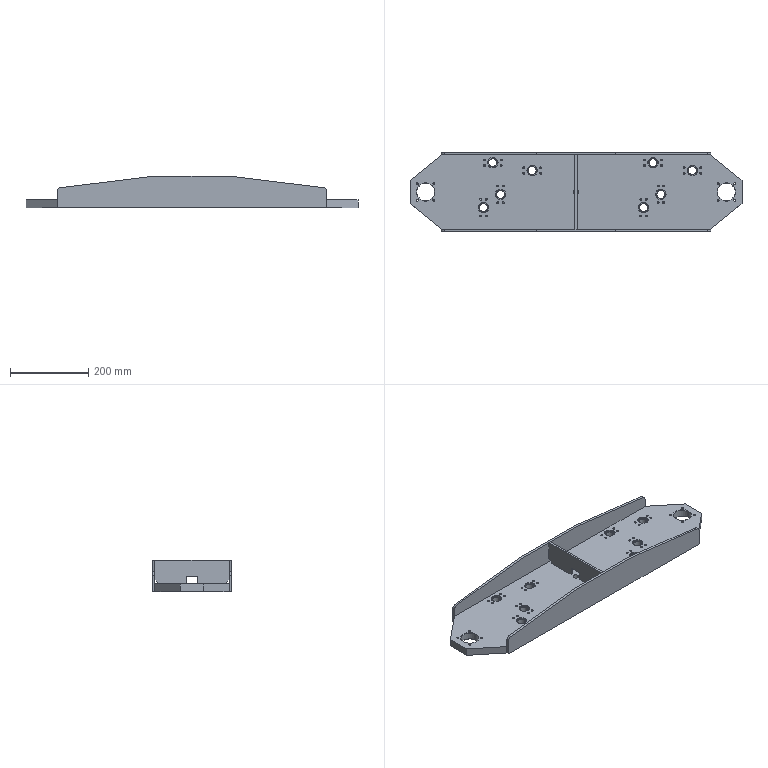Part | SolidWorks | features ICE 11, LPattern 6, 3DProfileFeature 4, HoleWzd 4, Chamfer 3, CirPattern 3, Extrusion 1, Fillet 1, MirrorPattern 1, MirrorSolid 1, WeldmentFeature 1 | 4 solids | 288 faces | box 850.5 x 202 x 80 mm | volume 3525282 mm3 | cylinder 122 | cone 120 | plane 46 | commonest cylinder face diameters 5 x80 20 x20 26 x16 45 x4 14.5 x2